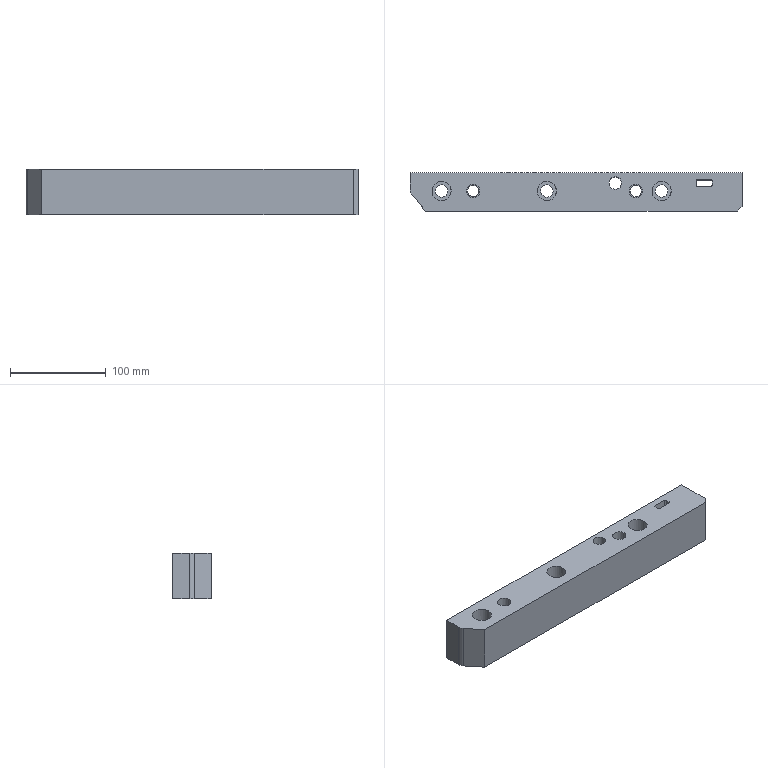Part | STEP file | gslz 2016.10.28-13_id1342_x_t | 1 solid | 33 faces | box 347 x 40 x 48 mm | volume 605773 mm3 | plane 17 | cylinder 16 | commonest cylinder face diameters 2 x4 13 x4 20 x3 12 x2 14 x2 18 x1